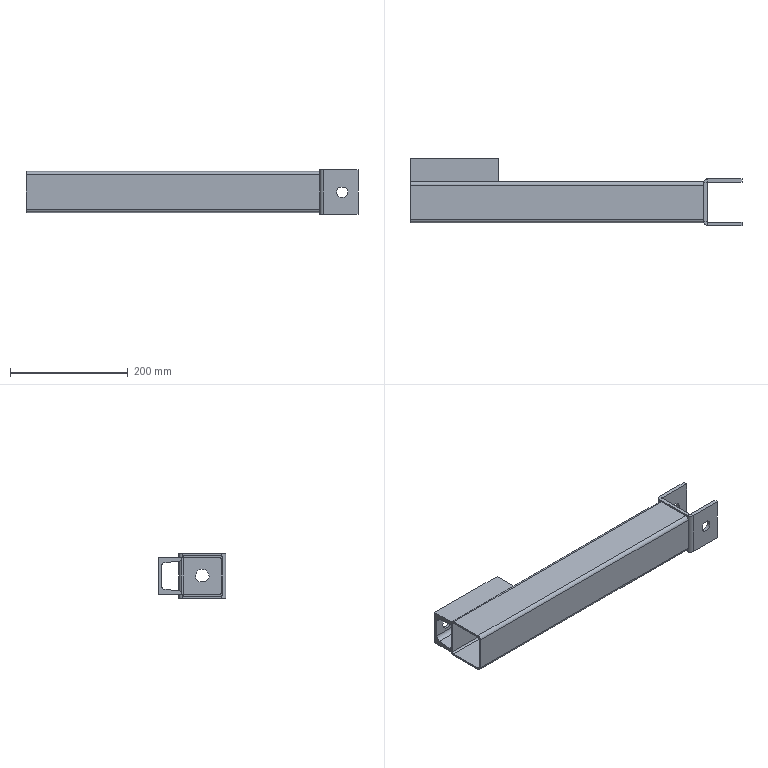Part | SolidWorks | features ICE 3, WeldMemberFeat 2, EdgeFlange 1, FlatPattern 1, SMBaseFlange 1, SheetMetal 1, WeldmentFeature 1 | 3 solids | 68 faces | box 565 x 115 x 75 mm | volume 595954 mm3 | plane 41 | cylinder 27 | commonest cylinder face diameters 19 x6 6 x4 12 x4 20 x4 1.473 x2 7.6 x2